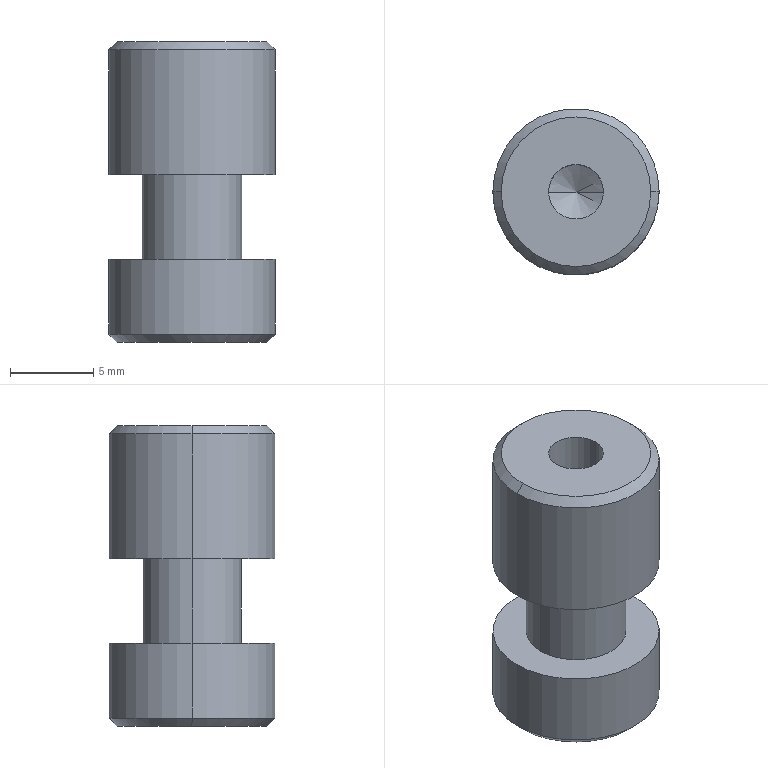Part | STEP file | 01-08 small floating joint | 1 solid | 18 faces | box 10 x 10 x 18.1 mm | volume 1056 mm3 | cylinder 8 | cone 6 | plane 4 | commonest cylinder face diameters 10 x4 3.3 x2 6 x2
STEP:
#1=CARTESIAN_POINT('',(-1.65,0.,6.6));
#2=VERTEX_POINT('',#1);
#3=CARTESIAN_POINT('',(1.65,0.,6.6));
#4=VERTEX_POINT('',#3);
#5=CARTESIAN_POINT('',(0.,0.,6.6));
#6=DIRECTION('',(0.,0.,1.));
#7=DIRECTION('',(1.,0.,0.));
#8=AXIS2_PLACEMENT_3D('',#5,#6,#7);
#9=CIRCLE('',#8,1.65);
#10=EDGE_CURVE('',#2,#4,#9,.T.);
#11=ORIENTED_EDGE('',*,*,#10,.F.);
#12=CARTESIAN_POINT('',(-1.65,0.,18.1));
#13=VERTEX_POINT('',#12);
#14=CARTESIAN_POINT('',(-1.65,0.,18.1));
#15=DIRECTION('',(0.,0.,1.));
#16=VECTOR('',#15,1000.);
#17=LINE('',#14,#16);
#18=EDGE_CURVE('',#2,#13,#17,.T.);
#19=ORIENTED_EDGE('',*,*,#18,.T.);
#20=CARTESIAN_POINT('',(1.65,0.,18.1));
#21=VERTEX_POINT('',#20);
#22=CARTESIAN_POINT('',(0.,0.,18.1));
#23=DIRECTION('',(0.,0.,1.));
#24=DIRECTION('',(1.,0.,0.));
#25=AXIS2_PLACEMENT_3D('',#22,#23,#24);
#26=CIRCLE('',#25,1.65);
#27=EDGE_CURVE('',#13,#21,#26,.T.);
#28=ORIENTED_EDGE('',*,*,#27,.T.);
#29=CARTESIAN_POINT('',(1.65,0.,18.1));
#30=DIRECTION('',(0.,0.,1.));
#31=VECTOR('',#30,1000.);
#32=LINE('',#29,#31);
#33=EDGE_CURVE('',#4,#21,#32,.T.);
#34=ORIENTED_EDGE('',*,*,#33,.F.);
#35=EDGE_LOOP('',(#11,#19,#28,#34));
#36=FACE_OUTER_BOUND('',#35,.T.);
#37=CARTESIAN_POINT('',(0.,0.,18.1));
#38=DIRECTION('',(0.,0.,1.));
#39=DIRECTION('',(1.,0.,0.));
#40=AXIS2_PLACEMENT_3D('',#37,#38,#39);
#41=CYLINDRICAL_SURFACE('',#40,1.65);
#42=ADVANCED_FACE('',(#36),#41,.F.);
#43=CARTESIAN_POINT('',(0.,0.,5.609));
#44=VERTEX_POINT('',#43);
#45=CARTESIAN_POINT('',(1.65,0.,6.6));
#46=DIRECTION('',(0.8572,0.,0.515));
#47=VECTOR('',#46,1000.);
#48=LINE('',#45,#47);
#49=EDGE_CURVE('',#44,#4,#48,.T.);
#50=ORIENTED_EDGE('',*,*,#49,.F.);
#51=CARTESIAN_POINT('',(-1.65,0.,6.6));
#52=DIRECTION('',(-0.8572,0.,0.515));
#53=VECTOR('',#52,1000.);
#54=LINE('',#51,#53);
#55=EDGE_CURVE('',#44,#2,#54,.T.);
#56=ORIENTED_EDGE('',*,*,#55,.T.);
#57=ORIENTED_EDGE('',*,*,#10,.T.);
#58=EDGE_LOOP('',(#50,#56,#57));
#59=FACE_OUTER_BOUND('',#58,.T.);
#60=CARTESIAN_POINT('',(0.,0.,6.6));
#61=DIRECTION('',(0.,0.,1.));
#62=DIRECTION('',(1.,0.,0.));
#63=AXIS2_PLACEMENT_3D('',#60,#61,#62);
#64=CONICAL_SURFACE('',#63,1.65,1.03);
#65=ADVANCED_FACE('',(#59),#64,.F.);
#66=CARTESIAN_POINT('',(-4.5,0.,0.));
#67=VERTEX_POINT('',#66);
#68=CARTESIAN_POINT('',(4.5,0.,0.));
#69=VERTEX_POINT('',#68);
#70=CARTESIAN_POINT('',(0.,0.,0.));
#71=DIRECTION('',(0.,0.,-1.));
#72=DIRECTION('',(1.,0.,0.));
#73=AXIS2_PLACEMENT_3D('',#70,#71,#72);
#74=CIRCLE('',#73,4.5);
#75=EDGE_CURVE('',#67,#69,#74,.T.);
#76=ORIENTED_EDGE('',*,*,#75,.F.);
#77=CARTESIAN_POINT('',(-5.,0.,0.5));
#78=VERTEX_POINT('',#77);
#79=CARTESIAN_POINT('',(-5.,0.,0.5));
#80=DIRECTION('',(-0.7071,0.,0.7071));
#81=VECTOR('',#80,1000.);
#82=LINE('',#79,#81);
#83=EDGE_CURVE('',#67,#78,#82,.T.);
#84=ORIENTED_EDGE('',*,*,#83,.T.);
#85=CARTESIAN_POINT('',(5.,0.,0.5));
#86=VERTEX_POINT('',#85);
#87=CARTESIAN_POINT('',(0.,0.,0.5));
#88=DIRECTION('',(0.,0.,1.));
#89=DIRECTION('',(1.,0.,0.));
#90=AXIS2_PLACEMENT_3D('',#87,#88,#89);
#91=CIRCLE('',#90,5.);
#92=EDGE_CURVE('',#86,#78,#91,.T.);
#93=ORIENTED_EDGE('',*,*,#92,.F.);
#94=CARTESIAN_POINT('',(5.,0.,0.5));
#95=DIRECTION('',(0.7071,0.,0.7071));
#96=VECTOR('',#95,1000.);
#97=LINE('',#94,#96);
#98=EDGE_CURVE('',#69,#86,#97,.T.);
#99=ORIENTED_EDGE('',*,*,#98,.F.);
#100=EDGE_LOOP('',(#76,#84,#93,#99));
#101=FACE_OUTER_BOUND('',#100,.T.);
#102=CARTESIAN_POINT('',(0.,0.,0.5));
#103=DIRECTION('',(0.,0.,1.));
#104=DIRECTION('',(1.,0.,0.));
#105=AXIS2_PLACEMENT_3D('',#102,#103,#104);
#106=CONICAL_SURFACE('',#105,5.,0.7854);
#107=ADVANCED_FACE('',(#101),#106,.T.);
#108=CARTESIAN_POINT('',(4.5,0.,18.1));
#109=VERTEX_POINT('',#108);
#110=CARTESIAN_POINT('',(-4.5,0.,18.1));
#111=VERTEX_POINT('',#110);
#112=CARTESIAN_POINT('',(0.,0.,18.1));
#113=DIRECTION('',(0.,0.,1.));
#114=DIRECTION('',(1.,0.,0.));
#115=AXIS2_PLACEMENT_3D('',#112,#113,#114);
#116=CIRCLE('',#115,4.5);
#117=EDGE_CURVE('',#109,#111,#116,.T.);
#118=ORIENTED_EDGE('',*,*,#117,.F.);
#119=CARTESIAN_POINT('',(5.,0.,17.6));
#120=VERTEX_POINT('',#119);
#121=CARTESIAN_POINT('',(4.5,0.,18.1));
#122=DIRECTION('',(0.7071,0.,-0.7071));
#123=VECTOR('',#122,1000.);
#124=LINE('',#121,#123);
#125=EDGE_CURVE('',#109,#120,#124,.T.);
#126=ORIENTED_EDGE('',*,*,#125,.T.);
#127=CARTESIAN_POINT('',(-5.,0.,17.6));
#128=VERTEX_POINT('',#127);
#129=CARTESIAN_POINT('',(0.,0.,17.6));
#130=DIRECTION('',(0.,0.,-1.));
#131=DIRECTION('',(1.,0.,0.));
#132=AXIS2_PLACEMENT_3D('',#129,#130,#131);
#133=CIRCLE('',#132,5.);
#134=EDGE_CURVE('',#128,#120,#133,.T.);
#135=ORIENTED_EDGE('',*,*,#134,.F.);
#136=CARTESIAN_POINT('',(-4.5,0.,18.1));
#137=DIRECTION('',(-0.7071,0.,-0.7071));
#138=VECTOR('',#137,1000.);
#139=LINE('',#136,#138);
#140=EDGE_CURVE('',#111,#128,#139,.T.);
#141=ORIENTED_EDGE('',*,*,#140,.F.);
#142=EDGE_LOOP('',(#118,#126,#135,#141));
#143=FACE_OUTER_BOUND('',#142,.T.);
#144=CARTESIAN_POINT('',(0.,0.,18.1));
#145=DIRECTION('',(0.,0.,-1.));
#146=DIRECTION('',(-1.,0.,0.));
#147=AXIS2_PLACEMENT_3D('',#144,#145,#146);
#148=CONICAL_SURFACE('',#147,4.5,0.7854);
#149=ADVANCED_FACE('',(#143),#148,.T.);
#150=ORIENTED_EDGE('',*,*,#134,.T.);
#151=CARTESIAN_POINT('',(5.,0.,10.1));
#152=VERTEX_POINT('',#151);
#153=CARTESIAN_POINT('',(5.,0.,18.1));
#154=DIRECTION('',(0.,0.,-1.));
#155=VECTOR('',#154,1000.);
#156=LINE('',#153,#155);
#157=EDGE_CURVE('',#120,#152,#156,.T.);
#158=ORIENTED_EDGE('',*,*,#157,.T.);
#159=CARTESIAN_POINT('',(-5.,0.,10.1));
#160=VERTEX_POINT('',#159);
#161=CARTESIAN_POINT('',(0.,0.,10.1));
#162=DIRECTION('',(0.,0.,1.));
#163=DIRECTION('',(1.,0.,0.));
#164=AXIS2_PLACEMENT_3D('',#161,#162,#163);
#165=CIRCLE('',#164,5.);
#166=EDGE_CURVE('',#152,#160,#165,.T.);
#167=ORIENTED_EDGE('',*,*,#166,.T.);
#168=CARTESIAN_POINT('',(-5.,0.,18.1));
#169=DIRECTION('',(0.,0.,-1.));
#170=VECTOR('',#169,1000.);
#171=LINE('',#168,#170);
#172=EDGE_CURVE('',#128,#160,#171,.T.);
#173=ORIENTED_EDGE('',*,*,#172,.F.);
#174=EDGE_LOOP('',(#150,#158,#167,#173));
#175=FACE_OUTER_BOUND('',#174,.T.);
#176=CARTESIAN_POINT('',(0.,0.,18.1));
#177=DIRECTION('',(0.,0.,-1.));
#178=DIRECTION('',(-1.,0.,0.));
#179=AXIS2_PLACEMENT_3D('',#176,#177,#178);
#180=CYLINDRICAL_SURFACE('',#179,5.);
#181=ADVANCED_FACE('',(#175),#180,.T.);
#182=CARTESIAN_POINT('',(3.,0.,10.1));
#183=VERTEX_POINT('',#182);
#184=CARTESIAN_POINT('',(-3.,0.,10.1));
#185=VERTEX_POINT('',#184);
#186=CARTESIAN_POINT('',(0.,0.,10.1));
#187=DIRECTION('',(0.,0.,1.));
#188=DIRECTION('',(1.,0.,0.));
#189=AXIS2_PLACEMENT_3D('',#186,#187,#188);
#190=CIRCLE('',#189,3.);
#191=EDGE_CURVE('',#183,#185,#190,.T.);
#192=ORIENTED_EDGE('',*,*,#191,.F.);
#193=CARTESIAN_POINT('',(3.,0.,5.));
#194=VERTEX_POINT('',#193);
#195=CARTESIAN_POINT('',(3.,0.,10.1));
#196=DIRECTION('',(0.,0.,-1.));
#197=VECTOR('',#196,1000.);
#198=LINE('',#195,#197);
#199=EDGE_CURVE('',#183,#194,#198,.T.);
#200=ORIENTED_EDGE('',*,*,#199,.T.);
#201=CARTESIAN_POINT('',(-3.,0.,5.));
#202=VERTEX_POINT('',#201);
#203=CARTESIAN_POINT('',(0.,0.,5.));
#204=DIRECTION('',(0.,0.,1.));
#205=DIRECTION('',(1.,0.,0.));
#206=AXIS2_PLACEMENT_3D('',#203,#204,#205);
#207=CIRCLE('',#206,3.);
#208=EDGE_CURVE('',#194,#202,#207,.T.);
#209=ORIENTED_EDGE('',*,*,#208,.T.);
#210=CARTESIAN_POINT('',(-3.,0.,10.1));
#211=DIRECTION('',(0.,0.,-1.));
#212=VECTOR('',#211,1000.);
#213=LINE('',#210,#212);
#214=EDGE_CURVE('',#185,#202,#213,.T.);
#215=ORIENTED_EDGE('',*,*,#214,.F.);
#216=EDGE_LOOP('',(#192,#200,#209,#215));
#217=FACE_OUTER_BOUND('',#216,.T.);
#218=CARTESIAN_POINT('',(0.,0.,10.1));
#219=DIRECTION('',(0.,0.,-1.));
#220=DIRECTION('',(-1.,0.,0.));
#221=AXIS2_PLACEMENT_3D('',#218,#219,#220);
#222=CYLINDRICAL_SURFACE('',#221,3.);
#223=ADVANCED_FACE('',(#217),#222,.T.);
#224=CARTESIAN_POINT('',(5.,0.,5.));
#225=VERTEX_POINT('',#224);
#226=CARTESIAN_POINT('',(-5.,0.,5.));
#227=VERTEX_POINT('',#226);
#228=CARTESIAN_POINT('',(0.,0.,5.));
#229=DIRECTION('',(0.,0.,1.));
#230=DIRECTION('',(1.,0.,0.));
#231=AXIS2_PLACEMENT_3D('',#228,#229,#230);
#232=CIRCLE('',#231,5.);
#233=EDGE_CURVE('',#225,#227,#232,.T.);
#234=ORIENTED_EDGE('',*,*,#233,.F.);
#235=CARTESIAN_POINT('',(5.,0.,5.));
#236=DIRECTION('',(0.,0.,-1.));
#237=VECTOR('',#236,1000.);
#238=LINE('',#235,#237);
#239=EDGE_CURVE('',#225,#86,#238,.T.);
#240=ORIENTED_EDGE('',*,*,#239,.T.);
#241=ORIENTED_EDGE('',*,*,#92,.T.);
#242=CARTESIAN_POINT('',(-5.,0.,5.));
#243=DIRECTION('',(0.,0.,-1.));
#244=VECTOR('',#243,1000.);
#245=LINE('',#242,#244);
#246=EDGE_CURVE('',#227,#78,#245,.T.);
#247=ORIENTED_EDGE('',*,*,#246,.F.);
#248=EDGE_LOOP('',(#234,#240,#241,#247));
#249=FACE_OUTER_BOUND('',#248,.T.);
#250=CARTESIAN_POINT('',(0.,0.,5.));
#251=DIRECTION('',(0.,0.,-1.));
#252=DIRECTION('',(-1.,0.,0.));
#253=AXIS2_PLACEMENT_3D('',#250,#251,#252);
#254=CYLINDRICAL_SURFACE('',#253,5.);
#255=ADVANCED_FACE('',(#249),#254,.T.);
#256=CARTESIAN_POINT('',(0.,0.,5.));
#257=DIRECTION('',(0.,0.,1.));
#258=DIRECTION('',(1.,0.,0.));
#259=AXIS2_PLACEMENT_3D('',#256,#257,#258);
#260=CIRCLE('',#259,5.);
#261=EDGE_CURVE('',#227,#225,#260,.T.);
#262=ORIENTED_EDGE('',*,*,#261,.T.);
#263=ORIENTED_EDGE('',*,*,#233,.T.);
#264=EDGE_LOOP('',(#262,#263));
#265=FACE_OUTER_BOUND('',#264,.T.);
#266=CARTESIAN_POINT('',(0.,0.,5.));
#267=DIRECTION('',(0.,0.,1.));
#268=DIRECTION('',(1.,0.,0.));
#269=AXIS2_PLACEMENT_3D('',#266,#267,#268);
#270=CIRCLE('',#269,3.);
#271=EDGE_CURVE('',#202,#194,#270,.T.);
#272=ORIENTED_EDGE('',*,*,#271,.F.);
#273=ORIENTED_EDGE('',*,*,#208,.F.);
#274=EDGE_LOOP('',(#272,#273));
#275=FACE_BOUND('',#274,.T.);
#276=CARTESIAN_POINT('',(0.,0.,5.));
#277=DIRECTION('',(0.,0.,1.));
#278=DIRECTION('',(1.,0.,0.));
#279=AXIS2_PLACEMENT_3D('',#276,#277,#278);
#280=PLANE('',#279);
#281=ADVANCED_FACE('',(#265,#275),#280,.T.);
#282=ORIENTED_EDGE('',*,*,#239,.F.);
#283=ORIENTED_EDGE('',*,*,#261,.F.);
#284=ORIENTED_EDGE('',*,*,#246,.T.);
#285=CARTESIAN_POINT('',(0.,0.,0.5));
#286=DIRECTION('',(0.,0.,1.));
#287=DIRECTION('',(1.,0.,0.));
#288=AXIS2_PLACEMENT_3D('',#285,#286,#287);
#289=CIRCLE('',#288,5.);
#290=EDGE_CURVE('',#78,#86,#289,.T.);
#291=ORIENTED_EDGE('',*,*,#290,.T.);
#292=EDGE_LOOP('',(#282,#283,#284,#291));
#293=FACE_OUTER_BOUND('',#292,.T.);
#294=CARTESIAN_POINT('',(0.,0.,5.));
#295=DIRECTION('',(0.,0.,-1.));
#296=DIRECTION('',(-1.,0.,0.));
#297=AXIS2_PLACEMENT_3D('',#294,#295,#296);
#298=CYLINDRICAL_SURFACE('',#297,5.);
#299=ADVANCED_FACE('',(#293),#298,.T.);
#300=CARTESIAN_POINT('',(0.,0.,0.));
#301=DIRECTION('',(0.,0.,-1.));
#302=DIRECTION('',(1.,0.,0.));
#303=AXIS2_PLACEMENT_3D('',#300,#301,#302);
#304=CIRCLE('',#303,4.5);
#305=EDGE_CURVE('',#69,#67,#304,.T.);
#306=ORIENTED_EDGE('',*,*,#305,.T.);
#307=ORIENTED_EDGE('',*,*,#75,.T.);
#308=EDGE_LOOP('',(#306,#307));
#309=FACE_OUTER_BOUND('',#308,.T.);
#310=CARTESIAN_POINT('',(0.,0.,0.));
#311=DIRECTION('',(0.,0.,1.));
#312=DIRECTION('',(1.,0.,0.));
#313=AXIS2_PLACEMENT_3D('',#310,#311,#312);
#314=PLANE('',#313);
#315=ADVANCED_FACE('',(#309),#314,.F.);
#316=ORIENTED_EDGE('',*,*,#199,.F.);
#317=CARTESIAN_POINT('',(0.,0.,10.1));
#318=DIRECTION('',(0.,0.,1.));
#319=DIRECTION('',(1.,0.,0.));
#320=AXIS2_PLACEMENT_3D('',#317,#318,#319);
#321=CIRCLE('',#320,3.);
#322=EDGE_CURVE('',#185,#183,#321,.T.);
#323=ORIENTED_EDGE('',*,*,#322,.F.);
#324=ORIENTED_EDGE('',*,*,#214,.T.);
#325=ORIENTED_EDGE('',*,*,#271,.T.);
#326=EDGE_LOOP('',(#316,#323,#324,#325));
#327=FACE_OUTER_BOUND('',#326,.T.);
#328=CARTESIAN_POINT('',(0.,0.,10.1));
#329=DIRECTION('',(0.,0.,-1.));
#330=DIRECTION('',(-1.,0.,0.));
#331=AXIS2_PLACEMENT_3D('',#328,#329,#330);
#332=CYLINDRICAL_SURFACE('',#331,3.);
#333=ADVANCED_FACE('',(#327),#332,.T.);
#334=CARTESIAN_POINT('',(0.,0.,10.1));
#335=DIRECTION('',(0.,0.,1.));
#336=DIRECTION('',(1.,0.,0.));
#337=AXIS2_PLACEMENT_3D('',#334,#335,#336);
#338=CIRCLE('',#337,5.);
#339=EDGE_CURVE('',#160,#152,#338,.T.);
#340=ORIENTED_EDGE('',*,*,#339,.F.);
#341=ORIENTED_EDGE('',*,*,#166,.F.);
#342=EDGE_LOOP('',(#340,#341));
#343=FACE_OUTER_BOUND('',#342,.T.);
#344=ORIENTED_EDGE('',*,*,#322,.T.);
#345=ORIENTED_EDGE('',*,*,#191,.T.);
#346=EDGE_LOOP('',(#344,#345));
#347=FACE_BOUND('',#346,.T.);
#348=CARTESIAN_POINT('',(0.,0.,10.1));
#349=DIRECTION('',(0.,0.,1.));
#350=DIRECTION('',(1.,0.,0.));
#351=AXIS2_PLACEMENT_3D('',#348,#349,#350);
#352=PLANE('',#351);
#353=ADVANCED_FACE('',(#343,#347),#352,.F.);
#354=ORIENTED_EDGE('',*,*,#157,.F.);
#355=CARTESIAN_POINT('',(0.,0.,17.6));
#356=DIRECTION('',(0.,0.,-1.));
#357=DIRECTION('',(1.,0.,0.));
#358=AXIS2_PLACEMENT_3D('',#355,#356,#357);
#359=CIRCLE('',#358,5.);
#360=EDGE_CURVE('',#120,#128,#359,.T.);
#361=ORIENTED_EDGE('',*,*,#360,.T.);
#362=ORIENTED_EDGE('',*,*,#172,.T.);
#363=ORIENTED_EDGE('',*,*,#339,.T.);
#364=EDGE_LOOP('',(#354,#361,#362,#363));
#365=FACE_OUTER_BOUND('',#364,.T.);
#366=CARTESIAN_POINT('',(0.,0.,18.1));
#367=DIRECTION('',(0.,0.,-1.));
#368=DIRECTION('',(-1.,0.,0.));
#369=AXIS2_PLACEMENT_3D('',#366,#367,#368);
#370=CYLINDRICAL_SURFACE('',#369,5.);
#371=ADVANCED_FACE('',(#365),#370,.T.);
#372=CARTESIAN_POINT('',(0.,0.,18.1));
#373=DIRECTION('',(0.,0.,1.));
#374=DIRECTION('',(1.,0.,0.));
#375=AXIS2_PLACEMENT_3D('',#372,#373,#374);
#376=CIRCLE('',#375,1.65);
#377=EDGE_CURVE('',#21,#13,#376,.T.);
#378=ORIENTED_EDGE('',*,*,#377,.F.);
#379=ORIENTED_EDGE('',*,*,#27,.F.);
#380=EDGE_LOOP('',(#378,#379));
#381=FACE_BOUND('',#380,.T.);
#382=CARTESIAN_POINT('',(0.,0.,18.1));
#383=DIRECTION('',(0.,0.,1.));
#384=DIRECTION('',(1.,0.,0.));
#385=AXIS2_PLACEMENT_3D('',#382,#383,#384);
#386=CIRCLE('',#385,4.5);
#387=EDGE_CURVE('',#111,#109,#386,.T.);
#388=ORIENTED_EDGE('',*,*,#387,.T.);
#389=ORIENTED_EDGE('',*,*,#117,.T.);
#390=EDGE_LOOP('',(#388,#389));
#391=FACE_OUTER_BOUND('',#390,.T.);
#392=CARTESIAN_POINT('',(0.,0.,18.1));
#393=DIRECTION('',(0.,0.,1.));
#394=DIRECTION('',(1.,0.,0.));
#395=AXIS2_PLACEMENT_3D('',#392,#393,#394);
#396=PLANE('',#395);
#397=ADVANCED_FACE('',(#381,#391),#396,.T.);
#398=ORIENTED_EDGE('',*,*,#125,.F.);
#399=ORIENTED_EDGE('',*,*,#387,.F.);
#400=ORIENTED_EDGE('',*,*,#140,.T.);
#401=ORIENTED_EDGE('',*,*,#360,.F.);
#402=EDGE_LOOP('',(#398,#399,#400,#401));
#403=FACE_OUTER_BOUND('',#402,.T.);
#404=CARTESIAN_POINT('',(0.,0.,18.1));
#405=DIRECTION('',(0.,0.,-1.));
#406=DIRECTION('',(-1.,0.,0.));
#407=AXIS2_PLACEMENT_3D('',#404,#405,#406);
#408=CONICAL_SURFACE('',#407,4.5,0.7854);
#409=ADVANCED_FACE('',(#403),#408,.T.);
#410=ORIENTED_EDGE('',*,*,#83,.F.);
#411=ORIENTED_EDGE('',*,*,#305,.F.);
#412=ORIENTED_EDGE('',*,*,#98,.T.);
#413=ORIENTED_EDGE('',*,*,#290,.F.);
#414=EDGE_LOOP('',(#410,#411,#412,#413));
#415=FACE_OUTER_BOUND('',#414,.T.);
#416=CARTESIAN_POINT('',(0.,0.,0.5));
#417=DIRECTION('',(0.,0.,1.));
#418=DIRECTION('',(1.,0.,0.));
#419=AXIS2_PLACEMENT_3D('',#416,#417,#418);
#420=CONICAL_SURFACE('',#419,5.,0.7854);
#421=ADVANCED_FACE('',(#415),#420,.T.);
#422=ORIENTED_EDGE('',*,*,#55,.F.);
#423=ORIENTED_EDGE('',*,*,#49,.T.);
#424=CARTESIAN_POINT('',(0.,0.,6.6));
#425=DIRECTION('',(0.,0.,1.));
#426=DIRECTION('',(1.,0.,0.));
#427=AXIS2_PLACEMENT_3D('',#424,#425,#426);
#428=CIRCLE('',#427,1.65);
#429=EDGE_CURVE('',#4,#2,#428,.T.);
#430=ORIENTED_EDGE('',*,*,#429,.T.);
#431=EDGE_LOOP('',(#422,#423,#430));
#432=FACE_OUTER_BOUND('',#431,.T.);
#433=CARTESIAN_POINT('',(0.,0.,6.6));
#434=DIRECTION('',(0.,0.,1.));
#435=DIRECTION('',(1.,0.,0.));
#436=AXIS2_PLACEMENT_3D('',#433,#434,#435);
#437=CONICAL_SURFACE('',#436,1.65,1.03);
#438=ADVANCED_FACE('',(#432),#437,.F.);
#439=ORIENTED_EDGE('',*,*,#18,.F.);
#440=ORIENTED_EDGE('',*,*,#429,.F.);
#441=ORIENTED_EDGE('',*,*,#33,.T.);
#442=ORIENTED_EDGE('',*,*,#377,.T.);
#443=EDGE_LOOP('',(#439,#440,#441,#442));
#444=FACE_OUTER_BOUND('',#443,.T.);
#445=CARTESIAN_POINT('',(0.,0.,18.1));
#446=DIRECTION('',(0.,0.,1.));
#447=DIRECTION('',(1.,0.,0.));
#448=AXIS2_PLACEMENT_3D('',#445,#446,#447);
#449=CYLINDRICAL_SURFACE('',#448,1.65);
#450=ADVANCED_FACE('',(#444),#449,.F.);
#451=CLOSED_SHELL('',(#42,#65,#107,#149,#181,#223,#255,#281,#299,#315,#333,#353,#371,#397,#409,#421,#438,#450));
#452=MANIFOLD_SOLID_BREP('',#451);
#453=CARTESIAN_POINT('',(0.,0.,0.));
#454=DIRECTION('',(0.,0.,1.));
#455=DIRECTION('',(1.,0.,0.));
#456=AXIS2_PLACEMENT_3D('',#453,#454,#455);
#457=(LENGTH_UNIT()NAMED_UNIT(*)SI_UNIT(.MILLI.,.METRE.));
#458=UNCERTAINTY_MEASURE_WITH_UNIT(LENGTH_MEASURE(0.00001),#457,'','');
#459=(NAMED_UNIT(*)PLANE_ANGLE_UNIT()SI_UNIT($,.RADIAN.));
#460=(NAMED_UNIT(*)SI_UNIT($,.STERADIAN.)SOLID_ANGLE_UNIT());
#461=(GEOMETRIC_REPRESENTATION_CONTEXT(3)GLOBAL_UNCERTAINTY_ASSIGNED_CONTEXT((#458))GLOBAL_UNIT_ASSIGNED_CONTEXT((#457,#459,#460))REPRESENTATION_CONTEXT('',''));
#462=ADVANCED_BREP_SHAPE_REPRESENTATION('',(#452,#456),#461);